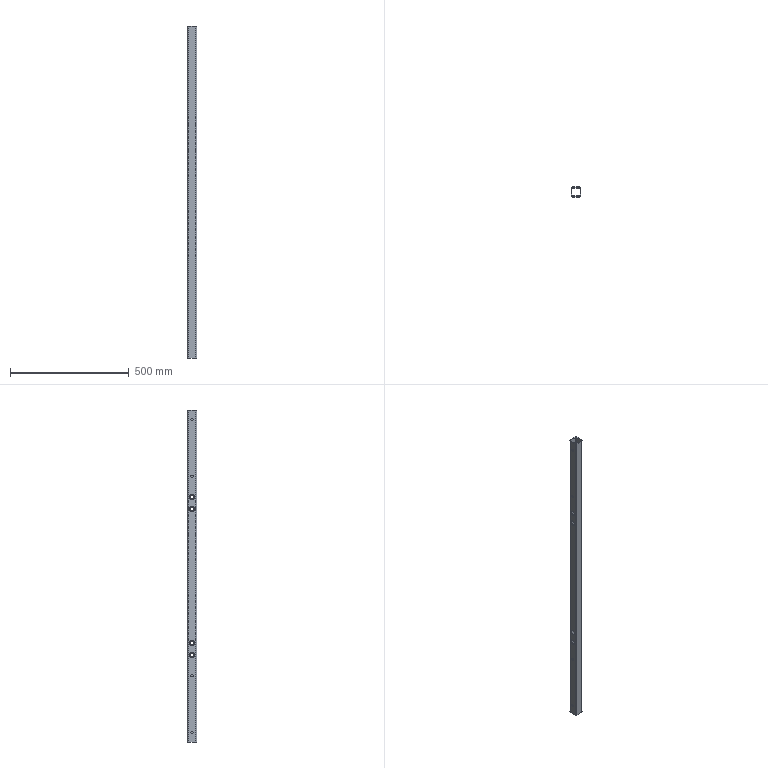Part | STEP file | DIN 59 410 - 40x40x2.9-800_DR_01 | 1 solid | 38 faces | box 40 x 40 x 1400 mm | volume 564745 mm3 | cylinder 20 | plane 10 | cone 8 | commonest cylinder face diameters 17.5 x8 5.8 x4 10 x4 11.6 x4